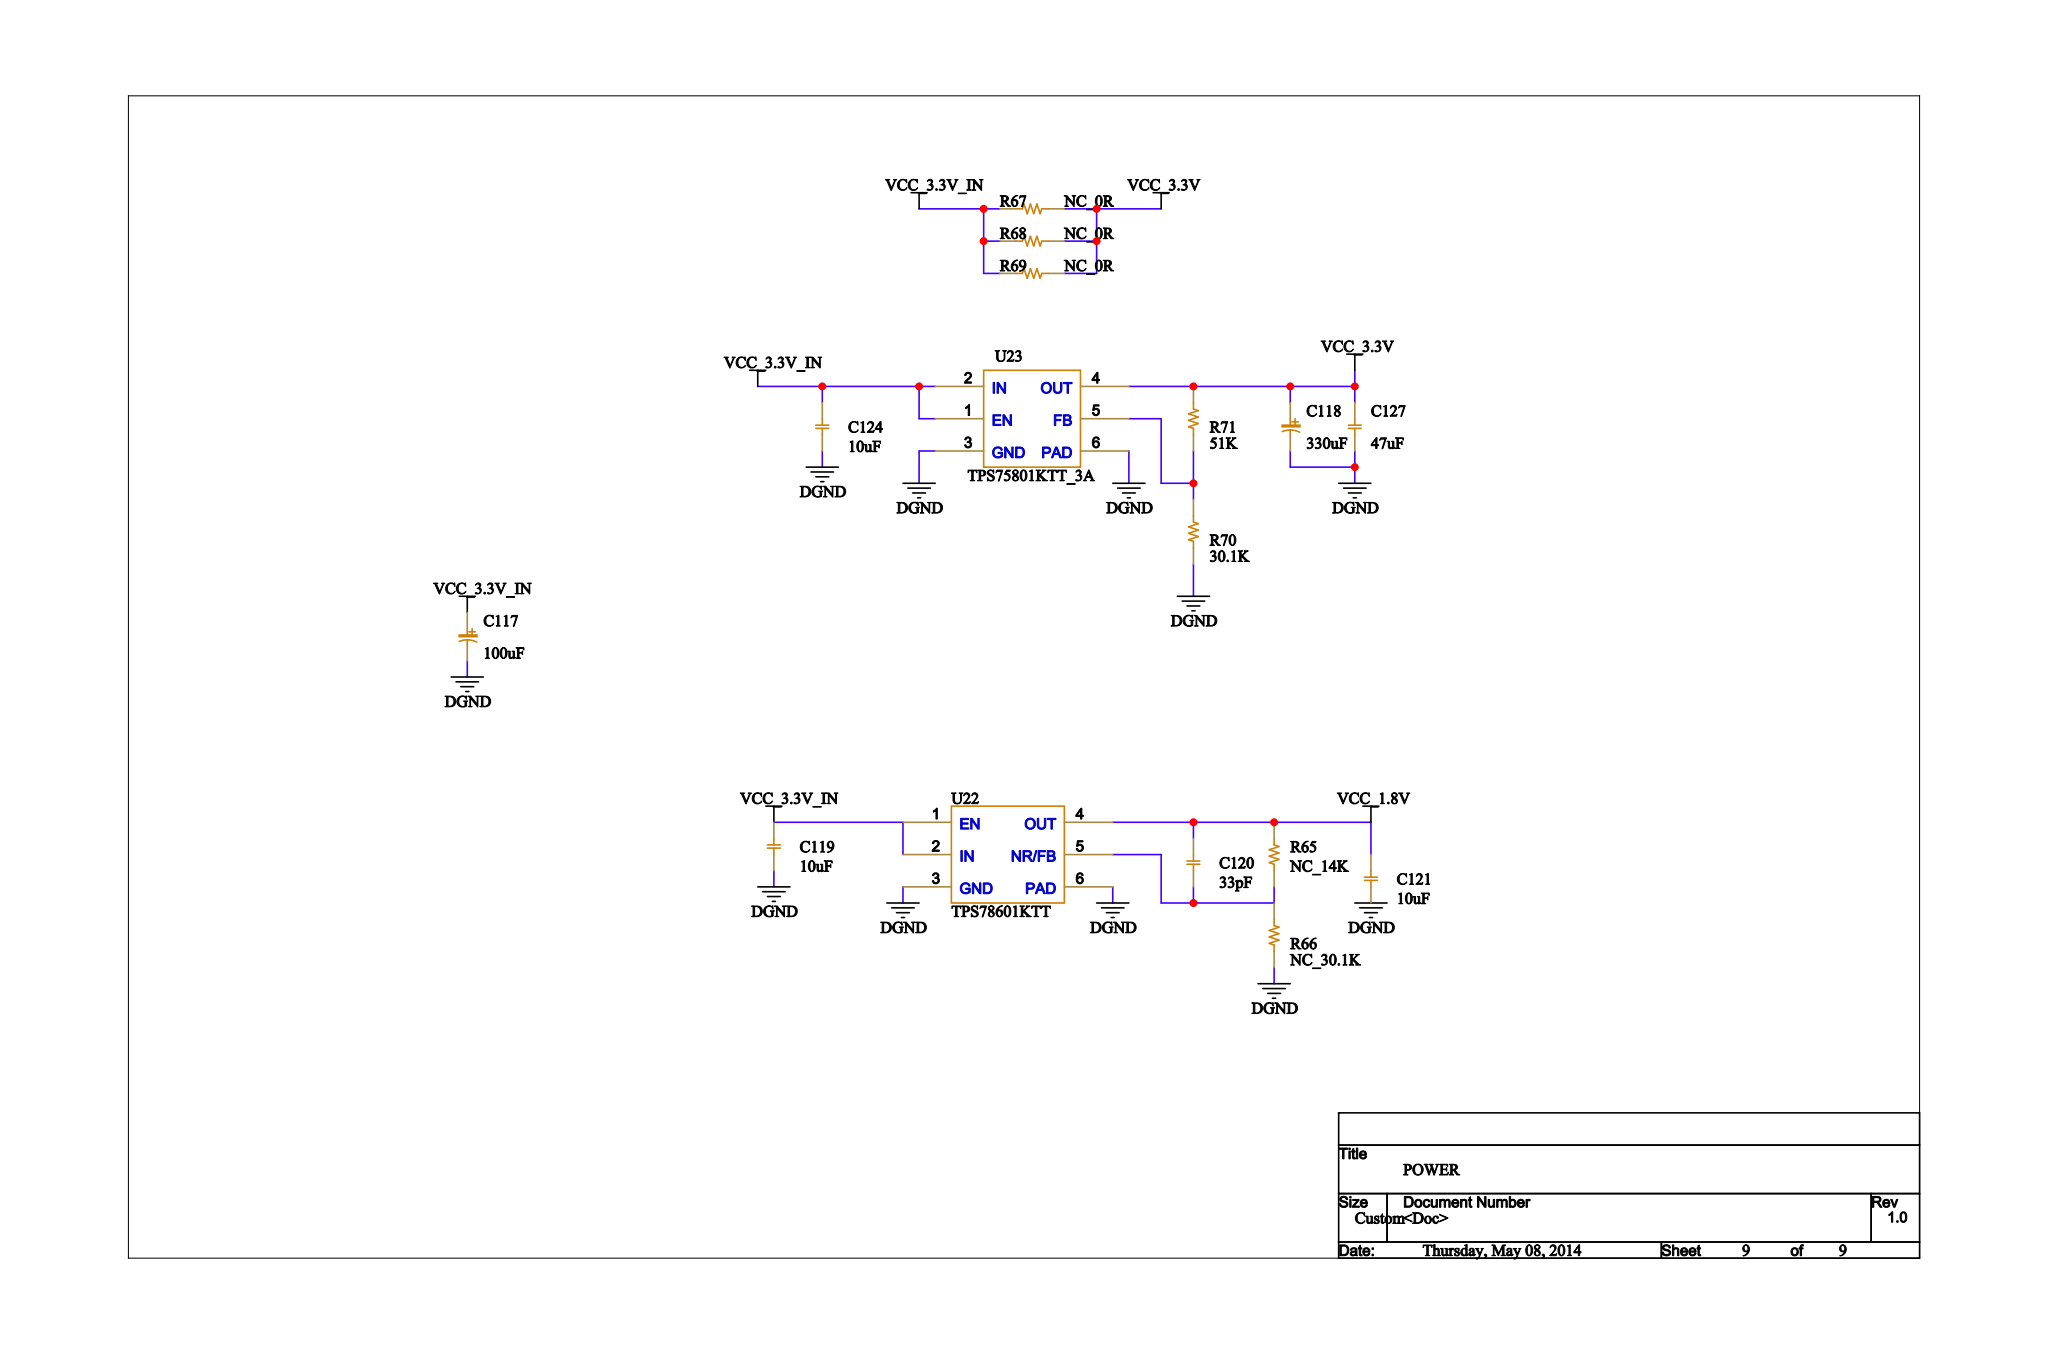Circuit board | Cadence Allegro | 233 parts | 224 nets | one sheet of the schematic
Parts on this sheet (reference | value | footprint):
C117 | 100uF | FPC-3528T
C118 | 330uF | FPC-7343T
C119 | 10uF | FPC-0603C
C120 | 33pF | FPC-0402C
C121 | 10uF | FPC-0603C
C124 | 10uF | FPC-0603C
C127 | 47uF | FPC-1206C
R65 | NC_14K | FPC-0603R
R66 | NC_30.1K | FPC-0603R
R67 | NC_0R | FPC-0603R
R68 | NC_0R | FPC-0603R
R69 | NC_0R | FPC-0603R
R70 | 30.1K | FPC-0603R
R71 | 51K | FPC-0603R
U22 | TPS78601KTT | FPC-TO-263
U23 | TPS75801KTT_3A | FPC-TO-263
Nets of these parts (net: part-pin ...):
DGND: C117-2 C118-2 C119-1 C121-1 C124-1 C127-2 R66-1 R70-1 U22-3 U22-6 U23-3 U23-6
VCC_3.3V: C118-1 C127-1 R67-1 R68-1 R69-1 R71-2 U23-4
VCC_1.8V: C120-2 C121-2 R65-2 U22-4
VCC_3.3V_IN: C117-1 C119-2 C124-2 R67-2 R68-2 R69-2 U22-1 U22-2 U23-1 U23-2
N571878: C120-1 R65-1 R66-2 U22-5
N549740: R70-2 R71-1 U23-5